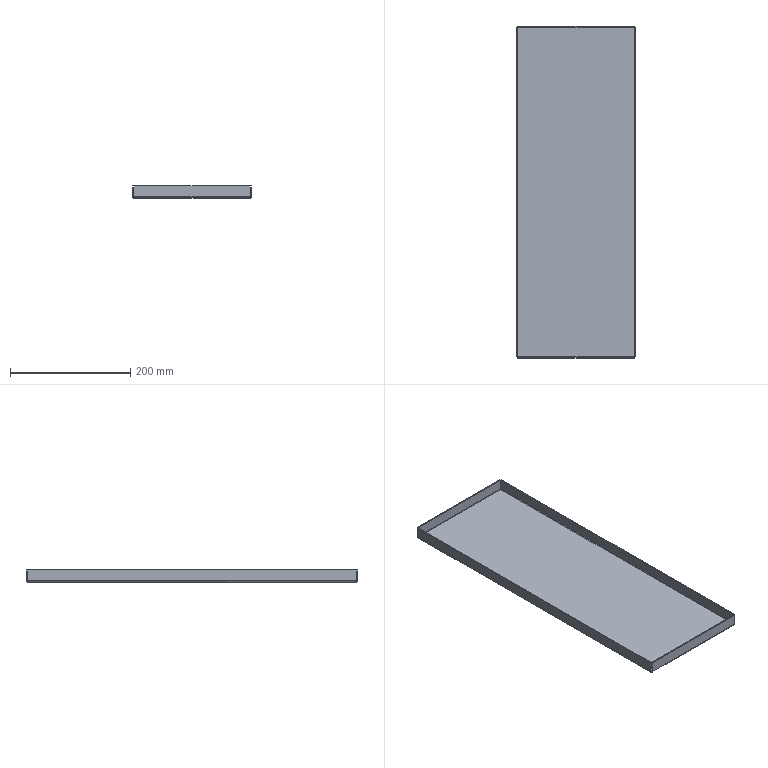Part | STEP file | X77-03021 | 1 solid | 38 faces | box 198 x 553 x 20 mm | volume 203981 mm3 | plane 22 | spline 8 | cylinder 8 | commonest cylinder face diameters 1.473 x4 4.473 x4